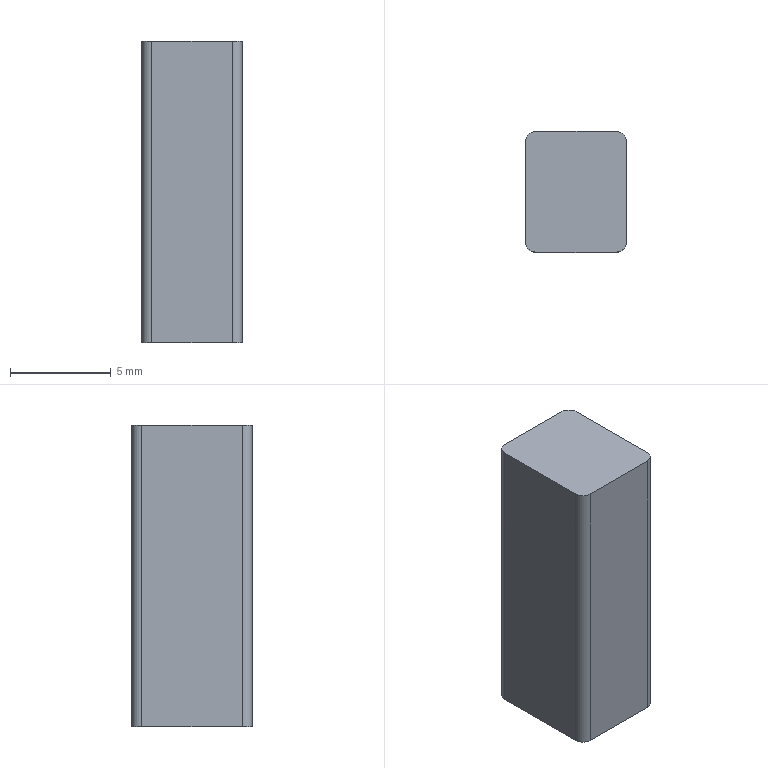Part | NX | features BREP 1 | 1 solid | 10 faces | box 5.02 x 6 x 15 mm | volume 448.59 mm3 | plane 6 | cylinder 4 | commonest cylinder face diameters 1 x4
STEP:
#1=CARTESIAN_POINT('',(-2.01,3.,-25.6));
#2=VERTEX_POINT('',#1);
#3=CARTESIAN_POINT('',(-2.51,2.5,-25.6));
#4=VERTEX_POINT('',#3);
#5=CARTESIAN_POINT('',(-2.01,2.5,-25.6));
#6=DIRECTION('',(0.,0.,1.));
#7=DIRECTION('',(1.,0.,0.));
#8=AXIS2_PLACEMENT_3D('',#5,#6,#7);
#9=CIRCLE('',#8,0.5);
#10=EDGE_CURVE('',#2,#4,#9,.T.);
#11=ORIENTED_EDGE('',*,*,#10,.F.);
#12=CARTESIAN_POINT('',(-2.01,3.,-40.6));
#13=VERTEX_POINT('',#12);
#14=CARTESIAN_POINT('',(-2.01,3.,-40.6));
#15=DIRECTION('',(0.,0.,1.));
#16=VECTOR('',#15,1000.);
#17=LINE('',#14,#16);
#18=EDGE_CURVE('',#13,#2,#17,.T.);
#19=ORIENTED_EDGE('',*,*,#18,.F.);
#20=CARTESIAN_POINT('',(-2.51,2.5,-40.6));
#21=VERTEX_POINT('',#20);
#22=CARTESIAN_POINT('',(-2.01,2.5,-40.6));
#23=DIRECTION('',(0.,0.,1.));
#24=DIRECTION('',(1.,0.,0.));
#25=AXIS2_PLACEMENT_3D('',#22,#23,#24);
#26=CIRCLE('',#25,0.5);
#27=EDGE_CURVE('',#13,#21,#26,.T.);
#28=ORIENTED_EDGE('',*,*,#27,.T.);
#29=CARTESIAN_POINT('',(-2.51,2.5,-40.6));
#30=DIRECTION('',(0.,0.,1.));
#31=VECTOR('',#30,1000.);
#32=LINE('',#29,#31);
#33=EDGE_CURVE('',#21,#4,#32,.T.);
#34=ORIENTED_EDGE('',*,*,#33,.T.);
#35=EDGE_LOOP('',(#11,#19,#28,#34));
#36=FACE_BOUND('',#35,.T.);
#37=CARTESIAN_POINT('',(-2.01,2.5,-40.6));
#38=DIRECTION('',(0.,0.,1.));
#39=DIRECTION('',(-1.,0.,0.));
#40=AXIS2_PLACEMENT_3D('',#37,#38,#39);
#41=CYLINDRICAL_SURFACE('',#40,0.5);
#42=ADVANCED_FACE('',(#36),#41,.T.);
#43=CARTESIAN_POINT('',(-2.51,-2.5,-25.6));
#44=VERTEX_POINT('',#43);
#45=CARTESIAN_POINT('',(-2.51,-2.5,-25.6));
#46=DIRECTION('',(0.,1.,0.));
#47=VECTOR('',#46,1000.);
#48=LINE('',#45,#47);
#49=EDGE_CURVE('',#44,#4,#48,.T.);
#50=ORIENTED_EDGE('',*,*,#49,.T.);
#51=ORIENTED_EDGE('',*,*,#33,.F.);
#52=CARTESIAN_POINT('',(-2.51,-2.5,-40.6));
#53=VERTEX_POINT('',#52);
#54=CARTESIAN_POINT('',(-2.51,-2.5,-40.6));
#55=DIRECTION('',(0.,1.,0.));
#56=VECTOR('',#55,1000.);
#57=LINE('',#54,#56);
#58=EDGE_CURVE('',#53,#21,#57,.T.);
#59=ORIENTED_EDGE('',*,*,#58,.F.);
#60=CARTESIAN_POINT('',(-2.51,-2.5,-40.6));
#61=DIRECTION('',(0.,0.,1.));
#62=VECTOR('',#61,1000.);
#63=LINE('',#60,#62);
#64=EDGE_CURVE('',#53,#44,#63,.T.);
#65=ORIENTED_EDGE('',*,*,#64,.T.);
#66=EDGE_LOOP('',(#50,#51,#59,#65));
#67=FACE_BOUND('',#66,.T.);
#68=CARTESIAN_POINT('',(-2.51,-2.5,-40.6));
#69=DIRECTION('',(1.,0.,0.));
#70=DIRECTION('',(0.,0.,1.));
#71=AXIS2_PLACEMENT_3D('',#68,#69,#70);
#72=PLANE('',#71);
#73=ADVANCED_FACE('',(#67),#72,.F.);
#74=CARTESIAN_POINT('',(-2.01,-3.,-25.6));
#75=VERTEX_POINT('',#74);
#76=CARTESIAN_POINT('',(-2.01,-2.5,-25.6));
#77=DIRECTION('',(0.,0.,1.));
#78=DIRECTION('',(1.,0.,0.));
#79=AXIS2_PLACEMENT_3D('',#76,#77,#78);
#80=CIRCLE('',#79,0.5);
#81=EDGE_CURVE('',#44,#75,#80,.T.);
#82=ORIENTED_EDGE('',*,*,#81,.F.);
#83=ORIENTED_EDGE('',*,*,#64,.F.);
#84=CARTESIAN_POINT('',(-2.01,-3.,-40.6));
#85=VERTEX_POINT('',#84);
#86=CARTESIAN_POINT('',(-2.01,-2.5,-40.6));
#87=DIRECTION('',(0.,0.,1.));
#88=DIRECTION('',(1.,0.,0.));
#89=AXIS2_PLACEMENT_3D('',#86,#87,#88);
#90=CIRCLE('',#89,0.5);
#91=EDGE_CURVE('',#53,#85,#90,.T.);
#92=ORIENTED_EDGE('',*,*,#91,.T.);
#93=CARTESIAN_POINT('',(-2.01,-3.,-40.6));
#94=DIRECTION('',(0.,0.,1.));
#95=VECTOR('',#94,1000.);
#96=LINE('',#93,#95);
#97=EDGE_CURVE('',#85,#75,#96,.T.);
#98=ORIENTED_EDGE('',*,*,#97,.T.);
#99=EDGE_LOOP('',(#82,#83,#92,#98));
#100=FACE_BOUND('',#99,.T.);
#101=CARTESIAN_POINT('',(-2.01,-2.5,-40.6));
#102=DIRECTION('',(0.,0.,1.));
#103=DIRECTION('',(-1.,0.,0.));
#104=AXIS2_PLACEMENT_3D('',#101,#102,#103);
#105=CYLINDRICAL_SURFACE('',#104,0.5);
#106=ADVANCED_FACE('',(#100),#105,.T.);
#107=CARTESIAN_POINT('',(2.01,-3.,-25.6));
#108=VERTEX_POINT('',#107);
#109=CARTESIAN_POINT('',(2.01,-3.,-25.6));
#110=DIRECTION('',(-1.,0.,0.));
#111=VECTOR('',#110,1000.);
#112=LINE('',#109,#111);
#113=EDGE_CURVE('',#108,#75,#112,.T.);
#114=ORIENTED_EDGE('',*,*,#113,.T.);
#115=ORIENTED_EDGE('',*,*,#97,.F.);
#116=CARTESIAN_POINT('',(2.01,-3.,-40.6));
#117=VERTEX_POINT('',#116);
#118=CARTESIAN_POINT('',(2.01,-3.,-40.6));
#119=DIRECTION('',(-1.,0.,0.));
#120=VECTOR('',#119,1000.);
#121=LINE('',#118,#120);
#122=EDGE_CURVE('',#117,#85,#121,.T.);
#123=ORIENTED_EDGE('',*,*,#122,.F.);
#124=CARTESIAN_POINT('',(2.01,-3.,-40.6));
#125=DIRECTION('',(0.,0.,1.));
#126=VECTOR('',#125,1000.);
#127=LINE('',#124,#126);
#128=EDGE_CURVE('',#117,#108,#127,.T.);
#129=ORIENTED_EDGE('',*,*,#128,.T.);
#130=EDGE_LOOP('',(#114,#115,#123,#129));
#131=FACE_BOUND('',#130,.T.);
#132=CARTESIAN_POINT('',(2.01,-3.,-40.6));
#133=DIRECTION('',(0.,1.,0.));
#134=DIRECTION('',(0.,0.,-1.));
#135=AXIS2_PLACEMENT_3D('',#132,#133,#134);
#136=PLANE('',#135);
#137=ADVANCED_FACE('',(#131),#136,.F.);
#138=CARTESIAN_POINT('',(2.51,-2.5,-25.6));
#139=VERTEX_POINT('',#138);
#140=CARTESIAN_POINT('',(2.01,-2.5,-25.6));
#141=DIRECTION('',(0.,0.,1.));
#142=DIRECTION('',(1.,0.,0.));
#143=AXIS2_PLACEMENT_3D('',#140,#141,#142);
#144=CIRCLE('',#143,0.5);
#145=EDGE_CURVE('',#108,#139,#144,.T.);
#146=ORIENTED_EDGE('',*,*,#145,.F.);
#147=ORIENTED_EDGE('',*,*,#128,.F.);
#148=CARTESIAN_POINT('',(2.51,-2.5,-40.6));
#149=VERTEX_POINT('',#148);
#150=CARTESIAN_POINT('',(2.01,-2.5,-40.6));
#151=DIRECTION('',(0.,0.,1.));
#152=DIRECTION('',(1.,0.,0.));
#153=AXIS2_PLACEMENT_3D('',#150,#151,#152);
#154=CIRCLE('',#153,0.5);
#155=EDGE_CURVE('',#117,#149,#154,.T.);
#156=ORIENTED_EDGE('',*,*,#155,.T.);
#157=CARTESIAN_POINT('',(2.51,-2.5,-40.6));
#158=DIRECTION('',(0.,0.,1.));
#159=VECTOR('',#158,1000.);
#160=LINE('',#157,#159);
#161=EDGE_CURVE('',#149,#139,#160,.T.);
#162=ORIENTED_EDGE('',*,*,#161,.T.);
#163=EDGE_LOOP('',(#146,#147,#156,#162));
#164=FACE_BOUND('',#163,.T.);
#165=CARTESIAN_POINT('',(2.01,-2.5,-40.6));
#166=DIRECTION('',(0.,0.,1.));
#167=DIRECTION('',(-1.,0.,0.));
#168=AXIS2_PLACEMENT_3D('',#165,#166,#167);
#169=CYLINDRICAL_SURFACE('',#168,0.5);
#170=ADVANCED_FACE('',(#164),#169,.T.);
#171=CARTESIAN_POINT('',(2.51,2.5,-25.6));
#172=VERTEX_POINT('',#171);
#173=CARTESIAN_POINT('',(2.51,2.5,-25.6));
#174=DIRECTION('',(0.,-1.,0.));
#175=VECTOR('',#174,1000.);
#176=LINE('',#173,#175);
#177=EDGE_CURVE('',#172,#139,#176,.T.);
#178=ORIENTED_EDGE('',*,*,#177,.T.);
#179=ORIENTED_EDGE('',*,*,#161,.F.);
#180=CARTESIAN_POINT('',(2.51,2.5,-40.6));
#181=VERTEX_POINT('',#180);
#182=CARTESIAN_POINT('',(2.51,2.5,-40.6));
#183=DIRECTION('',(0.,-1.,0.));
#184=VECTOR('',#183,1000.);
#185=LINE('',#182,#184);
#186=EDGE_CURVE('',#181,#149,#185,.T.);
#187=ORIENTED_EDGE('',*,*,#186,.F.);
#188=CARTESIAN_POINT('',(2.51,2.5,-40.6));
#189=DIRECTION('',(0.,0.,1.));
#190=VECTOR('',#189,1000.);
#191=LINE('',#188,#190);
#192=EDGE_CURVE('',#181,#172,#191,.T.);
#193=ORIENTED_EDGE('',*,*,#192,.T.);
#194=EDGE_LOOP('',(#178,#179,#187,#193));
#195=FACE_BOUND('',#194,.T.);
#196=CARTESIAN_POINT('',(2.51,2.5,-40.6));
#197=DIRECTION('',(-1.,0.,0.));
#198=DIRECTION('',(0.,0.,-1.));
#199=AXIS2_PLACEMENT_3D('',#196,#197,#198);
#200=PLANE('',#199);
#201=ADVANCED_FACE('',(#195),#200,.F.);
#202=CARTESIAN_POINT('',(2.01,3.,-25.6));
#203=VERTEX_POINT('',#202);
#204=CARTESIAN_POINT('',(2.01,2.5,-25.6));
#205=DIRECTION('',(0.,0.,1.));
#206=DIRECTION('',(1.,0.,0.));
#207=AXIS2_PLACEMENT_3D('',#204,#205,#206);
#208=CIRCLE('',#207,0.5);
#209=EDGE_CURVE('',#172,#203,#208,.T.);
#210=ORIENTED_EDGE('',*,*,#209,.F.);
#211=ORIENTED_EDGE('',*,*,#192,.F.);
#212=CARTESIAN_POINT('',(2.01,3.,-40.6));
#213=VERTEX_POINT('',#212);
#214=CARTESIAN_POINT('',(2.01,2.5,-40.6));
#215=DIRECTION('',(0.,0.,1.));
#216=DIRECTION('',(1.,0.,0.));
#217=AXIS2_PLACEMENT_3D('',#214,#215,#216);
#218=CIRCLE('',#217,0.5);
#219=EDGE_CURVE('',#181,#213,#218,.T.);
#220=ORIENTED_EDGE('',*,*,#219,.T.);
#221=CARTESIAN_POINT('',(2.01,3.,-40.6));
#222=DIRECTION('',(0.,0.,1.));
#223=VECTOR('',#222,1000.);
#224=LINE('',#221,#223);
#225=EDGE_CURVE('',#213,#203,#224,.T.);
#226=ORIENTED_EDGE('',*,*,#225,.T.);
#227=EDGE_LOOP('',(#210,#211,#220,#226));
#228=FACE_BOUND('',#227,.T.);
#229=CARTESIAN_POINT('',(2.01,2.5,-40.6));
#230=DIRECTION('',(0.,0.,1.));
#231=DIRECTION('',(-1.,0.,0.));
#232=AXIS2_PLACEMENT_3D('',#229,#230,#231);
#233=CYLINDRICAL_SURFACE('',#232,0.5);
#234=ADVANCED_FACE('',(#228),#233,.T.);
#235=CARTESIAN_POINT('',(-2.01,3.,-25.6));
#236=DIRECTION('',(1.,0.,0.));
#237=VECTOR('',#236,1000.);
#238=LINE('',#235,#237);
#239=EDGE_CURVE('',#2,#203,#238,.T.);
#240=ORIENTED_EDGE('',*,*,#239,.T.);
#241=ORIENTED_EDGE('',*,*,#225,.F.);
#242=CARTESIAN_POINT('',(-2.01,3.,-40.6));
#243=DIRECTION('',(1.,0.,0.));
#244=VECTOR('',#243,1000.);
#245=LINE('',#242,#244);
#246=EDGE_CURVE('',#13,#213,#245,.T.);
#247=ORIENTED_EDGE('',*,*,#246,.F.);
#248=ORIENTED_EDGE('',*,*,#18,.T.);
#249=EDGE_LOOP('',(#240,#241,#247,#248));
#250=FACE_BOUND('',#249,.T.);
#251=CARTESIAN_POINT('',(-2.01,3.,-40.6));
#252=DIRECTION('',(0.,-1.,0.));
#253=DIRECTION('',(0.,0.,1.));
#254=AXIS2_PLACEMENT_3D('',#251,#252,#253);
#255=PLANE('',#254);
#256=ADVANCED_FACE('',(#250),#255,.F.);
#257=ORIENTED_EDGE('',*,*,#27,.F.);
#258=ORIENTED_EDGE('',*,*,#246,.T.);
#259=ORIENTED_EDGE('',*,*,#219,.F.);
#260=ORIENTED_EDGE('',*,*,#186,.T.);
#261=ORIENTED_EDGE('',*,*,#155,.F.);
#262=ORIENTED_EDGE('',*,*,#122,.T.);
#263=ORIENTED_EDGE('',*,*,#91,.F.);
#264=ORIENTED_EDGE('',*,*,#58,.T.);
#265=EDGE_LOOP('',(#257,#258,#259,#260,#261,#262,#263,#264));
#266=FACE_BOUND('',#265,.T.);
#267=CARTESIAN_POINT('',(-2.01,2.5,-40.6));
#268=DIRECTION('',(0.,0.,1.));
#269=DIRECTION('',(-1.,0.,0.));
#270=AXIS2_PLACEMENT_3D('',#267,#268,#269);
#271=PLANE('',#270);
#272=ADVANCED_FACE('',(#266),#271,.F.);
#273=ORIENTED_EDGE('',*,*,#10,.T.);
#274=ORIENTED_EDGE('',*,*,#49,.F.);
#275=ORIENTED_EDGE('',*,*,#81,.T.);
#276=ORIENTED_EDGE('',*,*,#113,.F.);
#277=ORIENTED_EDGE('',*,*,#145,.T.);
#278=ORIENTED_EDGE('',*,*,#177,.F.);
#279=ORIENTED_EDGE('',*,*,#209,.T.);
#280=ORIENTED_EDGE('',*,*,#239,.F.);
#281=EDGE_LOOP('',(#273,#274,#275,#276,#277,#278,#279,#280));
#282=FACE_BOUND('',#281,.T.);
#283=CARTESIAN_POINT('',(-2.01,2.5,-25.6));
#284=DIRECTION('',(0.,0.,1.));
#285=DIRECTION('',(-1.,0.,0.));
#286=AXIS2_PLACEMENT_3D('',#283,#284,#285);
#287=PLANE('',#286);
#288=ADVANCED_FACE('',(#282),#287,.T.);
#289=CLOSED_SHELL('',(#42,#73,#106,#137,#170,#201,#234,#256,#272,#288));
#290=MANIFOLD_SOLID_BREP('',#289);
#291=(LENGTH_UNIT()NAMED_UNIT(*)SI_UNIT(.MILLI.,.METRE.));
#292=UNCERTAINTY_MEASURE_WITH_UNIT(LENGTH_MEASURE(0.00001),#291,'','');
#293=(NAMED_UNIT(*)PLANE_ANGLE_UNIT()SI_UNIT($,.RADIAN.));
#294=(NAMED_UNIT(*)SI_UNIT($,.STERADIAN.)SOLID_ANGLE_UNIT());
#295=(GEOMETRIC_REPRESENTATION_CONTEXT(3)GLOBAL_UNCERTAINTY_ASSIGNED_CONTEXT((#292))GLOBAL_UNIT_ASSIGNED_CONTEXT((#291,#293,#294))REPRESENTATION_CONTEXT('',''));
#296=ADVANCED_BREP_SHAPE_REPRESENTATION('',(#290),#295);